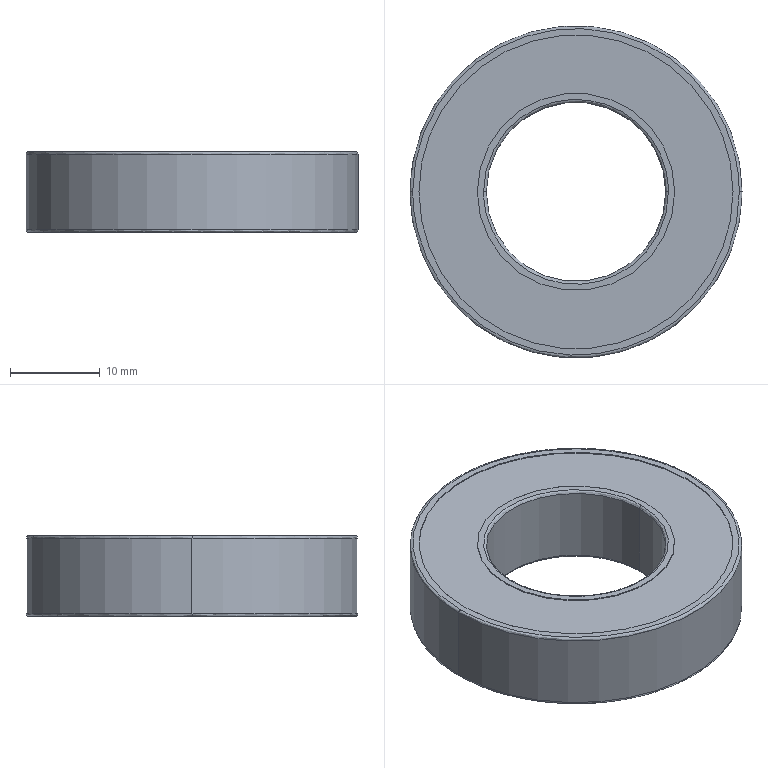Part | SolidWorks | features BaseBody 1 | 1 solid | 26 faces | box 37 x 37 x 9 mm | volume 6727 mm3 | cylinder 12 | spline 8 | plane 6 | commonest cylinder face diameters 22 x4 35 x4 20 x2 37 x2
STEP:
#1=CARTESIAN_POINT('',(-18.2,0.,-9.));
#2=VERTEX_POINT('',#1);
#3=CARTESIAN_POINT('',(18.2,0.,-9.));
#4=VERTEX_POINT('',#3);
#5=CARTESIAN_POINT('',(-18.2,0.,-9.));
#6=CARTESIAN_POINT('',(-18.2,-36.4,-9.));
#7=CARTESIAN_POINT('',(18.2,-36.4,-9.));
#8=CARTESIAN_POINT('',(18.2,0.,-9.));
#9=(BOUNDED_CURVE()B_SPLINE_CURVE(3,(#5,#6,#7,#8),.UNSPECIFIED.,.F.,.F.)B_SPLINE_CURVE_WITH_KNOTS((4,4),(0.,0.5),.UNSPECIFIED.)CURVE()GEOMETRIC_REPRESENTATION_ITEM()RATIONAL_B_SPLINE_CURVE((1.,0.3333,0.3333,1.))REPRESENTATION_ITEM(''));
#10=EDGE_CURVE('',#2,#4,#9,.T.);
#11=ORIENTED_EDGE('',*,*,#10,.T.);
#12=CARTESIAN_POINT('',(18.5,0.,-8.7));
#13=VERTEX_POINT('',#12);
#14=CARTESIAN_POINT('',(18.2,0.,-8.7));
#15=DIRECTION('',(0.,-1.,0.));
#16=DIRECTION('',(1.,0.,0.));
#17=AXIS2_PLACEMENT_3D('',#14,#15,#16);
#18=CIRCLE('',#17,0.3);
#19=EDGE_CURVE('',#4,#13,#18,.T.);
#20=ORIENTED_EDGE('',*,*,#19,.T.);
#21=CARTESIAN_POINT('',(-18.5,0.,-8.7));
#22=VERTEX_POINT('',#21);
#23=CARTESIAN_POINT('',(0.,0.,-8.7));
#24=DIRECTION('',(0.,0.,1.));
#25=DIRECTION('',(1.,0.,0.));
#26=AXIS2_PLACEMENT_3D('',#23,#24,#25);
#27=CIRCLE('',#26,18.5);
#28=EDGE_CURVE('',#22,#13,#27,.T.);
#29=ORIENTED_EDGE('',*,*,#28,.F.);
#30=CARTESIAN_POINT('',(-18.2,0.,-8.7));
#31=DIRECTION('',(0.,1.,0.));
#32=DIRECTION('',(-1.,0.,0.));
#33=AXIS2_PLACEMENT_3D('',#30,#31,#32);
#34=CIRCLE('',#33,0.3);
#35=EDGE_CURVE('',#2,#22,#34,.T.);
#36=ORIENTED_EDGE('',*,*,#35,.F.);
#37=EDGE_LOOP('',(#11,#20,#29,#36));
#38=FACE_OUTER_BOUND('',#37,.T.);
#39=CARTESIAN_POINT('',(18.2,0.,-9.));
#40=CARTESIAN_POINT('',(18.2,-36.4,-9.));
#41=CARTESIAN_POINT('',(-18.2,-36.4,-9.));
#42=CARTESIAN_POINT('',(-18.2,0.,-9.));
#43=CARTESIAN_POINT('',(18.376,0.,-9.));
#44=CARTESIAN_POINT('',(18.376,-36.751,-9.));
#45=CARTESIAN_POINT('',(-18.376,-36.751,-9.));
#46=CARTESIAN_POINT('',(-18.376,0.,-9.));
#47=CARTESIAN_POINT('',(18.5,0.,-8.876));
#48=CARTESIAN_POINT('',(18.5,-37.,-8.876));
#49=CARTESIAN_POINT('',(-18.5,-37.,-8.876));
#50=CARTESIAN_POINT('',(-18.5,0.,-8.876));
#51=CARTESIAN_POINT('',(18.5,0.,-8.7));
#52=CARTESIAN_POINT('',(18.5,-37.,-8.7));
#53=CARTESIAN_POINT('',(-18.5,-37.,-8.7));
#54=CARTESIAN_POINT('',(-18.5,0.,-8.7));
#55=(BOUNDED_SURFACE()B_SPLINE_SURFACE(3,3,((#39,#40,#41,#42),(#43,#44,#45,#46),(#47,#48,#49,#50),(#51,#52,#53,#54)),.UNSPECIFIED.,.F.,.F.,.F.)B_SPLINE_SURFACE_WITH_KNOTS((4,4),(4,4),(0.,1.),(0.,1.),.UNSPECIFIED.)GEOMETRIC_REPRESENTATION_ITEM()RATIONAL_B_SPLINE_SURFACE(((1.,0.3333,0.3333,1.),(0.8047,0.2682,0.2682,0.8047),(0.8047,0.2682,0.2682,0.8047),(1.,0.3333,0.3333,1.)))REPRESENTATION_ITEM('')SURFACE());
#56=ADVANCED_FACE('',(#38),#55,.T.);
#57=CARTESIAN_POINT('',(18.5,0.,-0.3));
#58=VERTEX_POINT('',#57);
#59=CARTESIAN_POINT('',(-18.5,0.,-0.3));
#60=VERTEX_POINT('',#59);
#61=CARTESIAN_POINT('',(0.,0.,-0.3));
#62=DIRECTION('',(0.,0.,-1.));
#63=DIRECTION('',(1.,0.,0.));
#64=AXIS2_PLACEMENT_3D('',#61,#62,#63);
#65=CIRCLE('',#64,18.5);
#66=EDGE_CURVE('',#58,#60,#65,.T.);
#67=ORIENTED_EDGE('',*,*,#66,.F.);
#68=CARTESIAN_POINT('',(18.2,0.,0.));
#69=VERTEX_POINT('',#68);
#70=CARTESIAN_POINT('',(18.2,0.,-0.3));
#71=DIRECTION('',(0.,-1.,0.));
#72=DIRECTION('',(1.,0.,0.));
#73=AXIS2_PLACEMENT_3D('',#70,#71,#72);
#74=CIRCLE('',#73,0.3);
#75=EDGE_CURVE('',#58,#69,#74,.T.);
#76=ORIENTED_EDGE('',*,*,#75,.T.);
#77=CARTESIAN_POINT('',(-18.2,0.,0.));
#78=VERTEX_POINT('',#77);
#79=CARTESIAN_POINT('',(18.2,0.,0.));
#80=CARTESIAN_POINT('',(18.2,-36.4,0.));
#81=CARTESIAN_POINT('',(-18.2,-36.4,0.));
#82=CARTESIAN_POINT('',(-18.2,0.,0.));
#83=(BOUNDED_CURVE()B_SPLINE_CURVE(3,(#79,#80,#81,#82),.UNSPECIFIED.,.F.,.F.)B_SPLINE_CURVE_WITH_KNOTS((4,4),(0.5,1.),.UNSPECIFIED.)CURVE()GEOMETRIC_REPRESENTATION_ITEM()RATIONAL_B_SPLINE_CURVE((1.,0.3333,0.3333,1.))REPRESENTATION_ITEM(''));
#84=EDGE_CURVE('',#69,#78,#83,.T.);
#85=ORIENTED_EDGE('',*,*,#84,.T.);
#86=CARTESIAN_POINT('',(-18.2,0.,-0.3));
#87=DIRECTION('',(0.,1.,0.));
#88=DIRECTION('',(-1.,0.,0.));
#89=AXIS2_PLACEMENT_3D('',#86,#87,#88);
#90=CIRCLE('',#89,0.3);
#91=EDGE_CURVE('',#60,#78,#90,.T.);
#92=ORIENTED_EDGE('',*,*,#91,.F.);
#93=EDGE_LOOP('',(#67,#76,#85,#92));
#94=FACE_OUTER_BOUND('',#93,.T.);
#95=CARTESIAN_POINT('',(18.5,0.,-0.3));
#96=CARTESIAN_POINT('',(18.5,-37.,-0.3));
#97=CARTESIAN_POINT('',(-18.5,-37.,-0.3));
#98=CARTESIAN_POINT('',(-18.5,0.,-0.3));
#99=CARTESIAN_POINT('',(18.5,0.,-0.1243));
#100=CARTESIAN_POINT('',(18.5,-37.,-0.1243));
#101=CARTESIAN_POINT('',(-18.5,-37.,-0.1243));
#102=CARTESIAN_POINT('',(-18.5,0.,-0.1243));
#103=CARTESIAN_POINT('',(18.376,0.,0.));
#104=CARTESIAN_POINT('',(18.376,-36.751,0.));
#105=CARTESIAN_POINT('',(-18.376,-36.751,0.));
#106=CARTESIAN_POINT('',(-18.376,0.,0.));
#107=CARTESIAN_POINT('',(18.2,0.,0.));
#108=CARTESIAN_POINT('',(18.2,-36.4,0.));
#109=CARTESIAN_POINT('',(-18.2,-36.4,0.));
#110=CARTESIAN_POINT('',(-18.2,0.,0.));
#111=(BOUNDED_SURFACE()B_SPLINE_SURFACE(3,3,((#95,#96,#97,#98),(#99,#100,#101,#102),(#103,#104,#105,#106),(#107,#108,#109,#110)),.UNSPECIFIED.,.F.,.F.,.F.)B_SPLINE_SURFACE_WITH_KNOTS((4,4),(4,4),(0.,1.),(0.,1.),.UNSPECIFIED.)GEOMETRIC_REPRESENTATION_ITEM()RATIONAL_B_SPLINE_SURFACE(((1.,0.3333,0.3333,1.),(0.8047,0.2682,0.2682,0.8047),(0.8047,0.2682,0.2682,0.8047),(1.,0.3333,0.3333,1.)))REPRESENTATION_ITEM('')SURFACE());
#112=ADVANCED_FACE('',(#94),#111,.T.);
#113=CARTESIAN_POINT('',(-10.,0.,-8.7));
#114=VERTEX_POINT('',#113);
#115=CARTESIAN_POINT('',(10.,0.,-8.7));
#116=VERTEX_POINT('',#115);
#117=CARTESIAN_POINT('',(0.,0.,-8.7));
#118=DIRECTION('',(0.,0.,1.));
#119=DIRECTION('',(-1.,0.,0.));
#120=AXIS2_PLACEMENT_3D('',#117,#118,#119);
#121=CIRCLE('',#120,10.);
#122=EDGE_CURVE('',#114,#116,#121,.T.);
#123=ORIENTED_EDGE('',*,*,#122,.T.);
#124=CARTESIAN_POINT('',(10.3,0.,-9.));
#125=VERTEX_POINT('',#124);
#126=CARTESIAN_POINT('',(10.3,0.,-8.7));
#127=DIRECTION('',(0.,-1.,0.));
#128=DIRECTION('',(1.,0.,0.));
#129=AXIS2_PLACEMENT_3D('',#126,#127,#128);
#130=CIRCLE('',#129,0.3);
#131=EDGE_CURVE('',#116,#125,#130,.T.);
#132=ORIENTED_EDGE('',*,*,#131,.T.);
#133=CARTESIAN_POINT('',(-10.3,0.,-9.));
#134=VERTEX_POINT('',#133);
#135=CARTESIAN_POINT('',(-10.3,0.,-9.));
#136=CARTESIAN_POINT('',(-10.3,-0.3149,-9.));
#137=CARTESIAN_POINT('',(-10.279,-0.7854,-9.));
#138=CARTESIAN_POINT('',(-10.216,-1.331,-9.));
#139=CARTESIAN_POINT('',(-10.175,-1.603,-9.));
#140=CARTESIAN_POINT('',(-10.152,-1.739,-9.));
#141=CARTESIAN_POINT('',(-10.142,-1.797,-9.));
#142=CARTESIAN_POINT('',(-10.135,-1.835,-9.));
#143=CARTESIAN_POINT('',(-10.132,-1.854,-9.));
#144=CARTESIAN_POINT('',(-10.067,-2.203,-9.));
#145=CARTESIAN_POINT('',(-9.953,-2.688,-9.));
#146=CARTESIAN_POINT('',(-9.778,-3.244,-9.));
#147=CARTESIAN_POINT('',(-9.681,-3.519,-9.));
#148=CARTESIAN_POINT('',(-9.637,-3.636,-9.));
#149=CARTESIAN_POINT('',(-9.607,-3.714,-9.));
#150=CARTESIAN_POINT('',(-9.593,-3.751,-9.));
#151=CARTESIAN_POINT('',(-9.449,-4.115,-9.));
#152=CARTESIAN_POINT('',(-9.233,-4.588,-9.));
#153=CARTESIAN_POINT('',(-8.941,-5.119,-9.));
#154=CARTESIAN_POINT('',(-8.807,-5.342,-9.));
#155=CARTESIAN_POINT('',(-8.715,-5.49,-9.));
#156=CARTESIAN_POINT('',(-8.67,-5.562,-9.));
#157=CARTESIAN_POINT('',(-8.232,-6.231,-9.));
#158=CARTESIAN_POINT('',(-7.786,-6.781,-9.));
#159=CARTESIAN_POINT('',(-7.032,-7.534,-9.));
#160=CARTESIAN_POINT('',(-6.638,-7.89,-9.));
#161=CARTESIAN_POINT('',(-6.147,-8.268,-9.));
#162=CARTESIAN_POINT('',(-5.93,-8.422,-9.));
#163=CARTESIAN_POINT('',(-5.784,-8.523,-9.));
#164=CARTESIAN_POINT('',(-5.709,-8.573,-9.));
#165=CARTESIAN_POINT('',(-5.345,-8.811,-9.));
#166=CARTESIAN_POINT('',(-4.896,-9.074,-9.));
#167=CARTESIAN_POINT('',(-4.351,-9.339,-9.));
#168=CARTESIAN_POINT('',(-4.073,-9.461,-9.));
#169=CARTESIAN_POINT('',(-3.953,-9.512,-9.));
#170=CARTESIAN_POINT('',(-3.872,-9.545,-9.));
#171=CARTESIAN_POINT('',(-3.83,-9.561,-9.));
#172=CARTESIAN_POINT('',(-3.481,-9.7,-9.));
#173=CARTESIAN_POINT('',(-3.008,-9.861,-9.));
#174=CARTESIAN_POINT('',(-2.445,-10.008,-9.));
#175=CARTESIAN_POINT('',(-2.161,-10.071,-9.));
#176=CARTESIAN_POINT('',(-2.018,-10.101,-9.));
#177=CARTESIAN_POINT('',(-1.956,-10.113,-9.));
#178=CARTESIAN_POINT('',(-1.915,-10.12,-9.));
#179=CARTESIAN_POINT('',(-1.894,-10.124,-9.));
#180=CARTESIAN_POINT('',(-1.255,-10.243,-9.));
#181=CARTESIAN_POINT('',(-0.6296,-10.3,-9.));
#182=CARTESIAN_POINT('',(0.3148,-10.3,-9.));
#183=CARTESIAN_POINT('',(0.7852,-10.279,-9.));
#184=CARTESIAN_POINT('',(1.331,-10.216,-9.));
#185=CARTESIAN_POINT('',(1.603,-10.175,-9.));
#186=CARTESIAN_POINT('',(1.739,-10.152,-9.));
#187=CARTESIAN_POINT('',(1.797,-10.142,-9.));
#188=CARTESIAN_POINT('',(1.835,-10.135,-9.));
#189=CARTESIAN_POINT('',(1.854,-10.132,-9.));
#190=CARTESIAN_POINT('',(2.203,-10.067,-9.));
#191=CARTESIAN_POINT('',(2.688,-9.953,-9.));
#192=CARTESIAN_POINT('',(3.244,-9.778,-9.));
#193=CARTESIAN_POINT('',(3.519,-9.681,-9.));
#194=CARTESIAN_POINT('',(3.636,-9.637,-9.));
#195=CARTESIAN_POINT('',(3.714,-9.607,-9.));
#196=CARTESIAN_POINT('',(3.751,-9.593,-9.));
#197=CARTESIAN_POINT('',(4.115,-9.449,-9.));
#198=CARTESIAN_POINT('',(4.588,-9.233,-9.));
#199=CARTESIAN_POINT('',(5.119,-8.941,-9.));
#200=CARTESIAN_POINT('',(5.342,-8.807,-9.));
#201=CARTESIAN_POINT('',(5.49,-8.715,-9.));
#202=CARTESIAN_POINT('',(5.562,-8.67,-9.));
#203=CARTESIAN_POINT('',(6.231,-8.232,-9.));
#204=CARTESIAN_POINT('',(6.781,-7.786,-9.));
#205=CARTESIAN_POINT('',(7.534,-7.032,-9.));
#206=CARTESIAN_POINT('',(7.89,-6.638,-9.));
#207=CARTESIAN_POINT('',(8.268,-6.147,-9.));
#208=CARTESIAN_POINT('',(8.422,-5.93,-9.));
#209=CARTESIAN_POINT('',(8.523,-5.784,-9.));
#210=CARTESIAN_POINT('',(8.573,-5.709,-9.));
#211=CARTESIAN_POINT('',(8.811,-5.345,-9.));
#212=CARTESIAN_POINT('',(9.074,-4.896,-9.));
#213=CARTESIAN_POINT('',(9.339,-4.351,-9.));
#214=CARTESIAN_POINT('',(9.461,-4.073,-9.));
#215=CARTESIAN_POINT('',(9.512,-3.953,-9.));
#216=CARTESIAN_POINT('',(9.545,-3.872,-9.));
#217=CARTESIAN_POINT('',(9.561,-3.83,-9.));
#218=CARTESIAN_POINT('',(9.7,-3.481,-9.));
#219=CARTESIAN_POINT('',(9.861,-3.008,-9.));
#220=CARTESIAN_POINT('',(10.008,-2.445,-9.));
#221=CARTESIAN_POINT('',(10.071,-2.161,-9.));
#222=CARTESIAN_POINT('',(10.101,-2.018,-9.));
#223=CARTESIAN_POINT('',(10.113,-1.956,-9.));
#224=CARTESIAN_POINT('',(10.12,-1.915,-9.));
#225=CARTESIAN_POINT('',(10.124,-1.894,-9.));
#226=CARTESIAN_POINT('',(10.243,-1.255,-9.));
#227=CARTESIAN_POINT('',(10.3,-0.6296,-9.));
#228=CARTESIAN_POINT('',(10.3,0.,-9.));
#229=B_SPLINE_CURVE_WITH_KNOTS('',3,(#135,#136,#137,#138,#139,#140,#141,#142,#143,#144,#145,#146,#147,#148,#149,#150,#151,#152,#153,#154,#155,#156,#157,#158,#159,#160,#161,#162,#163,#164,#165,#166,#167,#168,#169,#170,#171,#172,#173,#174,#175,#176,#177,#178,#179,#180,#181,#182,#183,#184,#185,#186,#187,#188,#189,#190,#191,#192,#193,#194,#195,#196,#197,#198,#199,#200,#201,#202,#203,#204,#205,#206,#207,#208,#209,#210,#211,#212,#213,#214,#215,#216,#217,#218,#219,#220,#221,#222,#223,#224,#225,#226,#227,#228),.UNSPECIFIED.,.F.,.F.,(4,1,1,1,1,2,2,1,1,1,2,2,1,1,2,2,2,1,1,2,2,1,1,1,2,2,1,1,1,1,2,2,2,1,1,1,1,2,2,1,1,1,2,2,1,1,2,2,2,1,1,2,2,1,1,1,2,2,1,1,1,1,2,2,4),(0.,0.01563,0.02344,0.02734,0.0293,0.03027,0.03125,0.04688,0.05469,0.05859,0.06055,0.0625,0.07813,0.08594,0.08984,0.09375,0.125,0.1406,0.1484,0.1523,0.1563,0.1719,0.1797,0.1836,0.1855,0.1875,0.2031,0.2109,0.2148,0.2168,0.2178,0.2188,0.25,0.2656,0.2734,0.2773,0.2793,0.2803,0.2813,0.2969,0.3047,0.3086,0.3105,0.3125,0.3281,0.3359,0.3398,0.3438,0.375,0.3906,0.3984,0.4023,0.4063,0.4219,0.4297,0.4336,0.4355,0.4375,0.4531,0.4609,0.4648,0.4668,0.4678,0.4688,0.5),.UNSPECIFIED.);
#230=EDGE_CURVE('',#134,#125,#229,.T.);
#231=ORIENTED_EDGE('',*,*,#230,.F.);
#232=CARTESIAN_POINT('',(-10.3,0.,-8.7));
#233=DIRECTION('',(0.,1.,0.));
#234=DIRECTION('',(-1.,0.,0.));
#235=AXIS2_PLACEMENT_3D('',#232,#233,#234);
#236=CIRCLE('',#235,0.3);
#237=EDGE_CURVE('',#114,#134,#236,.T.);
#238=ORIENTED_EDGE('',*,*,#237,.F.);
#239=EDGE_LOOP('',(#123,#132,#231,#238));
#240=FACE_OUTER_BOUND('',#239,.T.);
#241=CARTESIAN_POINT('',(10.,0.,-8.7));
#242=CARTESIAN_POINT('',(10.,-20.,-8.7));
#243=CARTESIAN_POINT('',(-10.,-20.,-8.7));
#244=CARTESIAN_POINT('',(-10.,0.,-8.7));
#245=CARTESIAN_POINT('',(10.,0.,-8.876));
#246=CARTESIAN_POINT('',(10.,-20.,-8.876));
#247=CARTESIAN_POINT('',(-10.,-20.,-8.876));
#248=CARTESIAN_POINT('',(-10.,0.,-8.876));
#249=CARTESIAN_POINT('',(10.124,0.,-9.));
#250=CARTESIAN_POINT('',(10.124,-20.249,-9.));
#251=CARTESIAN_POINT('',(-10.124,-20.249,-9.));
#252=CARTESIAN_POINT('',(-10.124,0.,-9.));
#253=CARTESIAN_POINT('',(10.3,0.,-9.));
#254=CARTESIAN_POINT('',(10.3,-20.6,-9.));
#255=CARTESIAN_POINT('',(-10.3,-20.6,-9.));
#256=CARTESIAN_POINT('',(-10.3,0.,-9.));
#257=(BOUNDED_SURFACE()B_SPLINE_SURFACE(3,3,((#241,#242,#243,#244),(#245,#246,#247,#248),(#249,#250,#251,#252),(#253,#254,#255,#256)),.UNSPECIFIED.,.F.,.F.,.F.)B_SPLINE_SURFACE_WITH_KNOTS((4,4),(4,4),(0.,1.),(0.,1.),.UNSPECIFIED.)GEOMETRIC_REPRESENTATION_ITEM()RATIONAL_B_SPLINE_SURFACE(((1.,0.3333,0.3333,1.),(0.8047,0.2682,0.2682,0.8047),(0.8047,0.2682,0.2682,0.8047),(1.,0.3333,0.3333,1.)))REPRESENTATION_ITEM('')SURFACE());
#258=ADVANCED_FACE('',(#240),#257,.T.);
#259=CARTESIAN_POINT('',(10.3,0.,0.));
#260=VERTEX_POINT('',#259);
#261=CARTESIAN_POINT('',(-10.3,0.,0.));
#262=VERTEX_POINT('',#261);
#263=CARTESIAN_POINT('',(10.3,0.,0.));
#264=CARTESIAN_POINT('',(10.3,-0.3148,0.));
#265=CARTESIAN_POINT('',(10.279,-0.7852,0.));
#266=CARTESIAN_POINT('',(10.216,-1.331,0.));
#267=CARTESIAN_POINT('',(10.175,-1.603,0.));
#268=CARTESIAN_POINT('',(10.152,-1.739,0.));
#269=CARTESIAN_POINT('',(10.142,-1.797,0.));
#270=CARTESIAN_POINT('',(10.135,-1.835,0.));
#271=CARTESIAN_POINT('',(10.132,-1.854,0.));
#272=CARTESIAN_POINT('',(10.067,-2.203,0.));
#273=CARTESIAN_POINT('',(9.953,-2.688,0.));
#274=CARTESIAN_POINT('',(9.778,-3.244,0.));
#275=CARTESIAN_POINT('',(9.681,-3.519,0.));
#276=CARTESIAN_POINT('',(9.637,-3.636,0.));
#277=CARTESIAN_POINT('',(9.607,-3.714,0.));
#278=CARTESIAN_POINT('',(9.593,-3.751,0.));
#279=CARTESIAN_POINT('',(9.449,-4.115,0.));
#280=CARTESIAN_POINT('',(9.233,-4.588,0.));
#281=CARTESIAN_POINT('',(8.941,-5.119,0.));
#282=CARTESIAN_POINT('',(8.807,-5.342,0.));
#283=CARTESIAN_POINT('',(8.715,-5.49,0.));
#284=CARTESIAN_POINT('',(8.67,-5.562,0.));
#285=CARTESIAN_POINT('',(8.232,-6.231,0.));
#286=CARTESIAN_POINT('',(7.786,-6.781,0.));
#287=CARTESIAN_POINT('',(7.032,-7.534,0.));
#288=CARTESIAN_POINT('',(6.638,-7.89,0.));
#289=CARTESIAN_POINT('',(6.147,-8.268,0.));
#290=CARTESIAN_POINT('',(5.93,-8.422,0.));
#291=CARTESIAN_POINT('',(5.784,-8.523,0.));
#292=CARTESIAN_POINT('',(5.709,-8.573,0.));
#293=CARTESIAN_POINT('',(5.345,-8.811,0.));
#294=CARTESIAN_POINT('',(4.896,-9.074,0.));
#295=CARTESIAN_POINT('',(4.351,-9.339,0.));
#296=CARTESIAN_POINT('',(4.073,-9.461,0.));
#297=CARTESIAN_POINT('',(3.953,-9.512,0.));
#298=CARTESIAN_POINT('',(3.872,-9.545,0.));
#299=CARTESIAN_POINT('',(3.83,-9.561,0.));
#300=CARTESIAN_POINT('',(3.481,-9.7,0.));
#301=CARTESIAN_POINT('',(3.008,-9.861,0.));
#302=CARTESIAN_POINT('',(2.445,-10.008,0.));
#303=CARTESIAN_POINT('',(2.161,-10.071,0.));
#304=CARTESIAN_POINT('',(2.018,-10.101,0.));
#305=CARTESIAN_POINT('',(1.956,-10.113,0.));
#306=CARTESIAN_POINT('',(1.915,-10.12,0.));
#307=CARTESIAN_POINT('',(1.894,-10.124,0.));
#308=CARTESIAN_POINT('',(1.255,-10.243,0.));
#309=CARTESIAN_POINT('',(0.6296,-10.3,0.));
#310=CARTESIAN_POINT('',(-0.3148,-10.3,0.));
#311=CARTESIAN_POINT('',(-0.7852,-10.279,0.));
#312=CARTESIAN_POINT('',(-1.331,-10.216,0.));
#313=CARTESIAN_POINT('',(-1.603,-10.175,0.));
#314=CARTESIAN_POINT('',(-1.739,-10.152,0.));
#315=CARTESIAN_POINT('',(-1.797,-10.142,0.));
#316=CARTESIAN_POINT('',(-1.835,-10.135,0.));
#317=CARTESIAN_POINT('',(-1.854,-10.132,0.));
#318=CARTESIAN_POINT('',(-2.203,-10.067,0.));
#319=CARTESIAN_POINT('',(-2.688,-9.953,0.));
#320=CARTESIAN_POINT('',(-3.244,-9.778,0.));
#321=CARTESIAN_POINT('',(-3.519,-9.681,0.));
#322=CARTESIAN_POINT('',(-3.636,-9.637,0.));
#323=CARTESIAN_POINT('',(-3.714,-9.607,0.));
#324=CARTESIAN_POINT('',(-3.751,-9.593,0.));
#325=CARTESIAN_POINT('',(-4.115,-9.449,0.));
#326=CARTESIAN_POINT('',(-4.588,-9.233,0.));
#327=CARTESIAN_POINT('',(-5.119,-8.941,0.));
#328=CARTESIAN_POINT('',(-5.342,-8.807,0.));
#329=CARTESIAN_POINT('',(-5.49,-8.715,0.));
#330=CARTESIAN_POINT('',(-5.562,-8.67,0.));
#331=CARTESIAN_POINT('',(-6.231,-8.232,0.));
#332=CARTESIAN_POINT('',(-6.781,-7.786,0.));
#333=CARTESIAN_POINT('',(-7.534,-7.032,0.));
#334=CARTESIAN_POINT('',(-7.89,-6.638,0.));
#335=CARTESIAN_POINT('',(-8.268,-6.147,0.));
#336=CARTESIAN_POINT('',(-8.422,-5.93,0.));
#337=CARTESIAN_POINT('',(-8.523,-5.784,0.));
#338=CARTESIAN_POINT('',(-8.573,-5.709,0.));
#339=CARTESIAN_POINT('',(-8.811,-5.345,0.));
#340=CARTESIAN_POINT('',(-9.074,-4.896,0.));
#341=CARTESIAN_POINT('',(-9.339,-4.351,0.));
#342=CARTESIAN_POINT('',(-9.461,-4.073,0.));
#343=CARTESIAN_POINT('',(-9.512,-3.953,0.));
#344=CARTESIAN_POINT('',(-9.545,-3.872,0.));
#345=CARTESIAN_POINT('',(-9.561,-3.83,0.));
#346=CARTESIAN_POINT('',(-9.7,-3.481,0.));
#347=CARTESIAN_POINT('',(-9.861,-3.008,0.));
#348=CARTESIAN_POINT('',(-10.008,-2.445,0.));
#349=CARTESIAN_POINT('',(-10.071,-2.161,0.));
#350=CARTESIAN_POINT('',(-10.101,-2.018,0.));
#351=CARTESIAN_POINT('',(-10.113,-1.956,0.));
#352=CARTESIAN_POINT('',(-10.12,-1.915,0.));
#353=CARTESIAN_POINT('',(-10.124,-1.894,0.));
#354=CARTESIAN_POINT('',(-10.243,-1.255,0.));
#355=CARTESIAN_POINT('',(-10.3,-0.6302,0.));
#356=CARTESIAN_POINT('',(-10.3,0.,0.));
#357=B_SPLINE_CURVE_WITH_KNOTS('',3,(#263,#264,#265,#266,#267,#268,#269,#270,#271,#272,#273,#274,#275,#276,#277,#278,#279,#280,#281,#282,#283,#284,#285,#286,#287,#288,#289,#290,#291,#292,#293,#294,#295,#296,#297,#298,#299,#300,#301,#302,#303,#304,#305,#306,#307,#308,#309,#310,#311,#312,#313,#314,#315,#316,#317,#318,#319,#320,#321,#322,#323,#324,#325,#326,#327,#328,#329,#330,#331,#332,#333,#334,#335,#336,#337,#338,#339,#340,#341,#342,#343,#344,#345,#346,#347,#348,#349,#350,#351,#352,#353,#354,#355,#356),.UNSPECIFIED.,.F.,.F.,(4,1,1,1,1,2,2,1,1,1,2,2,1,1,2,2,2,1,1,2,2,1,1,1,2,2,1,1,1,1,2,2,2,1,1,1,1,2,2,1,1,1,2,2,1,1,2,2,2,1,1,2,2,1,1,1,2,2,1,1,1,1,2,2,4),(0.5,0.5156,0.5234,0.5273,0.5293,0.5303,0.5313,0.5469,0.5547,0.5586,0.5605,0.5625,0.5781,0.5859,0.5898,0.5938,0.625,0.6406,0.6484,0.6523,0.6563,0.6719,0.6797,0.6836,0.6855,0.6875,0.7031,0.7109,0.7148,0.7168,0.7178,0.7188,0.75,0.7656,0.7734,0.7773,0.7793,0.7803,0.7813,0.7969,0.8047,0.8086,0.8105,0.8125,0.8281,0.8359,0.8398,0.8438,0.875,0.8906,0.8984,0.9023,0.9063,0.9219,0.9297,0.9336,0.9355,0.9375,0.9531,0.9609,0.9648,0.9668,0.9678,0.9688,1.),.UNSPECIFIED.);
#358=EDGE_CURVE('',#260,#262,#357,.T.);
#359=ORIENTED_EDGE('',*,*,#358,.F.);
#360=CARTESIAN_POINT('',(10.,0.,-0.3));
#361=VERTEX_POINT('',#360);
#362=CARTESIAN_POINT('',(10.3,0.,-0.3));
#363=DIRECTION('',(0.,-1.,0.));
#364=DIRECTION('',(1.,0.,0.));
#365=AXIS2_PLACEMENT_3D('',#362,#363,#364);
#366=CIRCLE('',#365,0.3);
#367=EDGE_CURVE('',#260,#361,#366,.T.);
#368=ORIENTED_EDGE('',*,*,#367,.T.);
#369=CARTESIAN_POINT('',(-10.,0.,-0.3));
#370=VERTEX_POINT('',#369);
#371=CARTESIAN_POINT('',(0.,0.,-0.3));
#372=DIRECTION('',(0.,0.,-1.));
#373=DIRECTION('',(-1.,0.,0.));
#374=AXIS2_PLACEMENT_3D('',#371,#372,#373);
#375=CIRCLE('',#374,10.);
#376=EDGE_CURVE('',#361,#370,#375,.T.);
#377=ORIENTED_EDGE('',*,*,#376,.T.);
#378=CARTESIAN_POINT('',(-10.3,0.,-0.3));
#379=DIRECTION('',(0.,1.,0.));
#380=DIRECTION('',(-1.,0.,0.));
#381=AXIS2_PLACEMENT_3D('',#378,#379,#380);
#382=CIRCLE('',#381,0.3);
#383=EDGE_CURVE('',#262,#370,#382,.T.);
#384=ORIENTED_EDGE('',*,*,#383,.F.);
#385=EDGE_LOOP('',(#359,#368,#377,#384));
#386=FACE_OUTER_BOUND('',#385,.T.);
#387=CARTESIAN_POINT('',(10.3,0.,0.));
#388=CARTESIAN_POINT('',(10.3,-20.6,0.));
#389=CARTESIAN_POINT('',(-10.3,-20.6,0.));
#390=CARTESIAN_POINT('',(-10.3,0.,0.));
#391=CARTESIAN_POINT('',(10.124,0.,0.));
#392=CARTESIAN_POINT('',(10.124,-20.249,0.));
#393=CARTESIAN_POINT('',(-10.124,-20.249,0.));
#394=CARTESIAN_POINT('',(-10.124,0.,0.));
#395=CARTESIAN_POINT('',(10.,0.,-0.1243));
#396=CARTESIAN_POINT('',(10.,-20.,-0.1243));
#397=CARTESIAN_POINT('',(-10.,-20.,-0.1243));
#398=CARTESIAN_POINT('',(-10.,0.,-0.1243));
#399=CARTESIAN_POINT('',(10.,0.,-0.3));
#400=CARTESIAN_POINT('',(10.,-20.,-0.3));
#401=CARTESIAN_POINT('',(-10.,-20.,-0.3));
#402=CARTESIAN_POINT('',(-10.,0.,-0.3));
#403=(BOUNDED_SURFACE()B_SPLINE_SURFACE(3,3,((#387,#388,#389,#390),(#391,#392,#393,#394),(#395,#396,#397,#398),(#399,#400,#401,#402)),.UNSPECIFIED.,.F.,.F.,.F.)B_SPLINE_SURFACE_WITH_KNOTS((4,4),(4,4),(0.,1.),(0.,1.),.UNSPECIFIED.)GEOMETRIC_REPRESENTATION_ITEM()RATIONAL_B_SPLINE_SURFACE(((1.,0.3333,0.3333,1.),(0.8047,0.2682,0.2682,0.8047),(0.8047,0.2682,0.2682,0.8047),(1.,0.3333,0.3333,1.)))REPRESENTATION_ITEM('')SURFACE());
#404=ADVANCED_FACE('',(#386),#403,.T.);
#405=CARTESIAN_POINT('',(0.,0.,-8.7));
#406=DIRECTION('',(0.,0.,1.));
#407=DIRECTION('',(1.,0.,0.));
#408=AXIS2_PLACEMENT_3D('',#405,#406,#407);
#409=CIRCLE('',#408,18.5);
#410=EDGE_CURVE('',#13,#22,#409,.T.);
#411=ORIENTED_EDGE('',*,*,#410,.T.);
#412=CARTESIAN_POINT('',(-18.5,0.,-9.));
#413=DIRECTION('',(0.,0.,1.));
#414=VECTOR('',#413,1000.);
#415=LINE('',#412,#414);
#416=EDGE_CURVE('',#22,#60,#415,.T.);
#417=ORIENTED_EDGE('',*,*,#416,.T.);
#418=CARTESIAN_POINT('',(0.,0.,-0.3));
#419=DIRECTION('',(0.,0.,-1.));
#420=DIRECTION('',(1.,0.,0.));
#421=AXIS2_PLACEMENT_3D('',#418,#419,#420);
#422=CIRCLE('',#421,18.5);
#423=EDGE_CURVE('',#60,#58,#422,.T.);
#424=ORIENTED_EDGE('',*,*,#423,.T.);
#425=CARTESIAN_POINT('',(18.5,0.,-9.));
#426=DIRECTION('',(0.,0.,1.));
#427=VECTOR('',#426,1000.);
#428=LINE('',#425,#427);
#429=EDGE_CURVE('',#13,#58,#428,.T.);
#430=ORIENTED_EDGE('',*,*,#429,.F.);
#431=EDGE_LOOP('',(#411,#417,#424,#430));
#432=FACE_OUTER_BOUND('',#431,.T.);
#433=CARTESIAN_POINT('',(0.,0.,-9.));
#434=DIRECTION('',(0.,0.,1.));
#435=DIRECTION('',(1.,0.,0.));
#436=AXIS2_PLACEMENT_3D('',#433,#434,#435);
#437=CYLINDRICAL_SURFACE('',#436,18.5);
#438=ADVANCED_FACE('',(#432),#437,.T.);
#439=CARTESIAN_POINT('',(-17.5,0.,-9.));
#440=VERTEX_POINT('',#439);
#441=CARTESIAN_POINT('',(17.5,0.,-9.));
#442=VERTEX_POINT('',#441);
#443=CARTESIAN_POINT('',(0.,0.,-9.));
#444=DIRECTION('',(0.,0.,1.));
#445=DIRECTION('',(1.,0.,0.));
#446=AXIS2_PLACEMENT_3D('',#443,#444,#445);
#447=CIRCLE('',#446,17.5);
#448=EDGE_CURVE('',#440,#442,#447,.T.);
#449=ORIENTED_EDGE('',*,*,#448,.F.);
#450=CARTESIAN_POINT('',(-17.5,0.,-8.9));
#451=VERTEX_POINT('',#450);
#452=CARTESIAN_POINT('',(-17.5,0.,-9.));
#453=DIRECTION('',(0.,0.,1.));
#454=VECTOR('',#453,1000.);
#455=LINE('',#452,#454);
#456=EDGE_CURVE('',#440,#451,#455,.T.);
#457=ORIENTED_EDGE('',*,*,#456,.T.);
#458=CARTESIAN_POINT('',(17.5,0.,-8.9));
#459=VERTEX_POINT('',#458);
#460=CARTESIAN_POINT('',(0.,0.,-8.9));
#461=DIRECTION('',(0.,0.,-1.));
#462=DIRECTION('',(1.,0.,0.));
#463=AXIS2_PLACEMENT_3D('',#460,#461,#462);
#464=CIRCLE('',#463,17.5);
#465=EDGE_CURVE('',#459,#451,#464,.T.);
#466=ORIENTED_EDGE('',*,*,#465,.F.);
#467=CARTESIAN_POINT('',(17.5,0.,-9.));
#468=DIRECTION('',(0.,0.,1.));
#469=VECTOR('',#468,1000.);
#470=LINE('',#467,#469);
#471=EDGE_CURVE('',#442,#459,#470,.T.);
#472=ORIENTED_EDGE('',*,*,#471,.F.);
#473=EDGE_LOOP('',(#449,#457,#466,#472));
#474=FACE_OUTER_BOUND('',#473,.T.);
#475=CARTESIAN_POINT('',(0.,0.,-9.));
#476=DIRECTION('',(0.,0.,1.));
#477=DIRECTION('',(1.,0.,0.));
#478=AXIS2_PLACEMENT_3D('',#475,#476,#477);
#479=CYLINDRICAL_SURFACE('',#478,17.5);
#480=ADVANCED_FACE('',(#474),#479,.F.);
#481=CARTESIAN_POINT('',(-17.5,0.,-0.1));
#482=VERTEX_POINT('',#481);
#483=CARTESIAN_POINT('',(17.5,0.,-0.1));
#484=VERTEX_POINT('',#483);
#485=CARTESIAN_POINT('',(0.,0.,-0.1));
#486=DIRECTION('',(0.,0.,1.));
#487=DIRECTION('',(1.,0.,0.));
#488=AXIS2_PLACEMENT_3D('',#485,#486,#487);
#489=CIRCLE('',#488,17.5);
#490=EDGE_CURVE('',#482,#484,#489,.T.);
#491=ORIENTED_EDGE('',*,*,#490,.F.);
#492=CARTESIAN_POINT('',(-17.5,0.,0.));
#493=VERTEX_POINT('',#492);
#494=CARTESIAN_POINT('',(-17.5,0.,-9.));
#495=DIRECTION('',(0.,0.,1.));
#496=VECTOR('',#495,1000.);
#497=LINE('',#494,#496);
#498=EDGE_CURVE('',#482,#493,#497,.T.);
#499=ORIENTED_EDGE('',*,*,#498,.T.);
#500=CARTESIAN_POINT('',(17.5,0.,0.));
#501=VERTEX_POINT('',#500);
#502=CARTESIAN_POINT('',(0.,0.,0.));
#503=DIRECTION('',(0.,0.,-1.));
#504=DIRECTION('',(1.,0.,0.));
#505=AXIS2_PLACEMENT_3D('',#502,#503,#504);
#506=CIRCLE('',#505,17.5);
#507=EDGE_CURVE('',#501,#493,#506,.T.);
#508=ORIENTED_EDGE('',*,*,#507,.F.);
#509=CARTESIAN_POINT('',(17.5,0.,-9.));
#510=DIRECTION('',(0.,0.,1.));
#511=VECTOR('',#510,1000.);
#512=LINE('',#509,#511);
#513=EDGE_CURVE('',#484,#501,#512,.T.);
#514=ORIENTED_EDGE('',*,*,#513,.F.);
#515=EDGE_LOOP('',(#491,#499,#508,#514));
#516=FACE_OUTER_BOUND('',#515,.T.);
#517=CARTESIAN_POINT('',(0.,0.,-9.));
#518=DIRECTION('',(0.,0.,1.));
#519=DIRECTION('',(1.,0.,0.));
#520=AXIS2_PLACEMENT_3D('',#517,#518,#519);
#521=CYLINDRICAL_SURFACE('',#520,17.5);
#522=ADVANCED_FACE('',(#516),#521,.F.);
#523=CARTESIAN_POINT('',(11.,0.,-9.));
#524=VERTEX_POINT('',#523);
#525=CARTESIAN_POINT('',(-11.,0.,-9.));
#526=VERTEX_POINT('',#525);
#527=CARTESIAN_POINT('',(0.,0.,-9.));
#528=DIRECTION('',(0.,0.,1.));
#529=DIRECTION('',(1.,0.,0.));
#530=AXIS2_PLACEMENT_3D('',#527,#528,#529);
#531=CIRCLE('',#530,11.);
#532=EDGE_CURVE('',#524,#526,#531,.T.);
#533=ORIENTED_EDGE('',*,*,#532,.T.);
#534=CARTESIAN_POINT('',(-11.,0.,-8.9));
#535=VERTEX_POINT('',#534);
#536=CARTESIAN_POINT('',(-11.,0.,-9.));
#537=DIRECTION('',(0.,0.,1.));
#538=VECTOR('',#537,1000.);
#539=LINE('',#536,#538);
#540=EDGE_CURVE('',#526,#535,#539,.T.);
#541=ORIENTED_EDGE('',*,*,#540,.T.);
#542=CARTESIAN_POINT('',(11.,0.,-8.9));
#543=VERTEX_POINT('',#542);
#544=CARTESIAN_POINT('',(0.,0.,-8.9));
#545=DIRECTION('',(0.,0.,1.));
#546=DIRECTION('',(1.,0.,0.));
#547=AXIS2_PLACEMENT_3D('',#544,#545,#546);
#548=CIRCLE('',#547,11.);
#549=EDGE_CURVE('',#543,#535,#548,.T.);
#550=ORIENTED_EDGE('',*,*,#549,.F.);
#551=CARTESIAN_POINT('',(11.,0.,-9.));
#552=DIRECTION('',(0.,0.,1.));
#553=VECTOR('',#552,1000.);
#554=LINE('',#551,#553);
#555=EDGE_CURVE('',#524,#543,#554,.T.);
#556=ORIENTED_EDGE('',*,*,#555,.F.);
#557=EDGE_LOOP('',(#533,#541,#550,#556));
#558=FACE_OUTER_BOUND('',#557,.T.);
#559=CARTESIAN_POINT('',(0.,0.,-9.));
#560=DIRECTION('',(0.,0.,1.));
#561=DIRECTION('',(1.,0.,0.));
#562=AXIS2_PLACEMENT_3D('',#559,#560,#561);
#563=CYLINDRICAL_SURFACE('',#562,11.);
#564=ADVANCED_FACE('',(#558),#563,.T.);
#565=CARTESIAN_POINT('',(-11.,0.,-0.1));
#566=VERTEX_POINT('',#565);
#567=CARTESIAN_POINT('',(11.,0.,-0.1));
#568=VERTEX_POINT('',#567);
#569=CARTESIAN_POINT('',(0.,0.,-0.1));
#570=DIRECTION('',(0.,0.,-1.));
#571=DIRECTION('',(1.,0.,0.));
#572=AXIS2_PLACEMENT_3D('',#569,#570,#571);
#573=CIRCLE('',#572,11.);
#574=EDGE_CURVE('',#566,#568,#573,.T.);
#575=ORIENTED_EDGE('',*,*,#574,.F.);
#576=CARTESIAN_POINT('',(-11.,0.,0.));
#577=VERTEX_POINT('',#576);
#578=CARTESIAN_POINT('',(-11.,0.,-9.));
#579=DIRECTION('',(0.,0.,1.));
#580=VECTOR('',#579,1000.);
#581=LINE('',#578,#580);
#582=EDGE_CURVE('',#566,#577,#581,.T.);
#583=ORIENTED_EDGE('',*,*,#582,.T.);
#584=CARTESIAN_POINT('',(11.,0.,0.));
#585=VERTEX_POINT('',#584);
#586=CARTESIAN_POINT('',(0.,0.,0.));
#587=DIRECTION('',(0.,0.,-1.));
#588=DIRECTION('',(1.,0.,0.));
#589=AXIS2_PLACEMENT_3D('',#586,#587,#588);
#590=CIRCLE('',#589,11.);
#591=EDGE_CURVE('',#577,#585,#590,.T.);
#592=ORIENTED_EDGE('',*,*,#591,.T.);
#593=CARTESIAN_POINT('',(11.,0.,-9.));
#594=DIRECTION('',(0.,0.,1.));
#595=VECTOR('',#594,1000.);
#596=LINE('',#593,#595);
#597=EDGE_CURVE('',#568,#585,#596,.T.);
#598=ORIENTED_EDGE('',*,*,#597,.F.);
#599=EDGE_LOOP('',(#575,#583,#592,#598));
#600=FACE_OUTER_BOUND('',#599,.T.);
#601=CARTESIAN_POINT('',(0.,0.,-9.));
#602=DIRECTION('',(0.,0.,1.));
#603=DIRECTION('',(1.,0.,0.));
#604=AXIS2_PLACEMENT_3D('',#601,#602,#603);
#605=CYLINDRICAL_SURFACE('',#604,11.);
#606=ADVANCED_FACE('',(#600),#605,.T.);
#607=ORIENTED_EDGE('',*,*,#122,.F.);
#608=CARTESIAN_POINT('',(-10.,0.,-9.));
#609=DIRECTION('',(0.,0.,1.));
#610=VECTOR('',#609,1000.);
#611=LINE('',#608,#610);
#612=EDGE_CURVE('',#114,#370,#611,.T.);
#613=ORIENTED_EDGE('',*,*,#612,.T.);
#614=ORIENTED_EDGE('',*,*,#376,.F.);
#615=CARTESIAN_POINT('',(10.,0.,-9.));
#616=DIRECTION('',(0.,0.,1.));
#617=VECTOR('',#616,1000.);
#618=LINE('',#615,#617);
#619=EDGE_CURVE('',#116,#361,#618,.T.);
#620=ORIENTED_EDGE('',*,*,#619,.F.);
#621=EDGE_LOOP('',(#607,#613,#614,#620));
#622=FACE_OUTER_BOUND('',#621,.T.);
#623=CARTESIAN_POINT('',(0.,0.,-9.));
#624=DIRECTION('',(0.,0.,1.));
#625=DIRECTION('',(1.,0.,0.));
#626=AXIS2_PLACEMENT_3D('',#623,#624,#625);
#627=CYLINDRICAL_SURFACE('',#626,10.);
#628=ADVANCED_FACE('',(#622),#627,.F.);
#629=ORIENTED_EDGE('',*,*,#416,.F.);
#630=ORIENTED_EDGE('',*,*,#28,.T.);
#631=ORIENTED_EDGE('',*,*,#429,.T.);
#632=ORIENTED_EDGE('',*,*,#66,.T.);
#633=EDGE_LOOP('',(#629,#630,#631,#632));
#634=FACE_OUTER_BOUND('',#633,.T.);
#635=CARTESIAN_POINT('',(0.,0.,-9.));
#636=DIRECTION('',(0.,0.,1.));
#637=DIRECTION('',(1.,0.,0.));
#638=AXIS2_PLACEMENT_3D('',#635,#636,#637);
#639=CYLINDRICAL_SURFACE('',#638,18.5);
#640=ADVANCED_FACE('',(#634),#639,.T.);
#641=ORIENTED_EDGE('',*,*,#19,.F.);
#642=CARTESIAN_POINT('',(18.2,0.,-9.));
#643=CARTESIAN_POINT('',(18.2,36.4,-9.));
#644=CARTESIAN_POINT('',(-18.2,36.4,-9.));
#645=CARTESIAN_POINT('',(-18.2,0.,-9.));
#646=(BOUNDED_CURVE()B_SPLINE_CURVE(3,(#642,#643,#644,#645),.UNSPECIFIED.,.F.,.F.)B_SPLINE_CURVE_WITH_KNOTS((4,4),(0.5,1.),.UNSPECIFIED.)CURVE()GEOMETRIC_REPRESENTATION_ITEM()RATIONAL_B_SPLINE_CURVE((1.,0.3333,0.3333,1.))REPRESENTATION_ITEM(''));
#647=EDGE_CURVE('',#4,#2,#646,.T.);
#648=ORIENTED_EDGE('',*,*,#647,.T.);
#649=ORIENTED_EDGE('',*,*,#35,.T.);
#650=ORIENTED_EDGE('',*,*,#410,.F.);
#651=EDGE_LOOP('',(#641,#648,#649,#650));
#652=FACE_OUTER_BOUND('',#651,.T.);
#653=CARTESIAN_POINT('',(-18.2,0.,-9.));
#654=CARTESIAN_POINT('',(-18.2,36.4,-9.));
#655=CARTESIAN_POINT('',(18.2,36.4,-9.));
#656=CARTESIAN_POINT('',(18.2,0.,-9.));
#657=CARTESIAN_POINT('',(-18.376,0.,-9.));
#658=CARTESIAN_POINT('',(-18.376,36.751,-9.));
#659=CARTESIAN_POINT('',(18.376,36.751,-9.));
#660=CARTESIAN_POINT('',(18.376,0.,-9.));
#661=CARTESIAN_POINT('',(-18.5,0.,-8.876));
#662=CARTESIAN_POINT('',(-18.5,37.,-8.876));
#663=CARTESIAN_POINT('',(18.5,37.,-8.876));
#664=CARTESIAN_POINT('',(18.5,0.,-8.876));
#665=CARTESIAN_POINT('',(-18.5,0.,-8.7));
#666=CARTESIAN_POINT('',(-18.5,37.,-8.7));
#667=CARTESIAN_POINT('',(18.5,37.,-8.7));
#668=CARTESIAN_POINT('',(18.5,0.,-8.7));
#669=(BOUNDED_SURFACE()B_SPLINE_SURFACE(3,3,((#653,#654,#655,#656),(#657,#658,#659,#660),(#661,#662,#663,#664),(#665,#666,#667,#668)),.UNSPECIFIED.,.F.,.F.,.F.)B_SPLINE_SURFACE_WITH_KNOTS((4,4),(4,4),(0.,1.),(0.,1.),.UNSPECIFIED.)GEOMETRIC_REPRESENTATION_ITEM()RATIONAL_B_SPLINE_SURFACE(((1.,0.3333,0.3333,1.),(0.8047,0.2682,0.2682,0.8047),(0.8047,0.2682,0.2682,0.8047),(1.,0.3333,0.3333,1.)))REPRESENTATION_ITEM('')SURFACE());
#670=ADVANCED_FACE('',(#652),#669,.T.);
#671=ORIENTED_EDGE('',*,*,#75,.F.);
#672=ORIENTED_EDGE('',*,*,#423,.F.);
#673=ORIENTED_EDGE('',*,*,#91,.T.);
#674=CARTESIAN_POINT('',(-18.2,0.,0.));
#675=CARTESIAN_POINT('',(-18.2,36.4,0.));
#676=CARTESIAN_POINT('',(18.2,36.4,0.));
#677=CARTESIAN_POINT('',(18.2,0.,0.));
#678=(BOUNDED_CURVE()B_SPLINE_CURVE(3,(#674,#675,#676,#677),.UNSPECIFIED.,.F.,.F.)B_SPLINE_CURVE_WITH_KNOTS((4,4),(0.,0.5),.UNSPECIFIED.)CURVE()GEOMETRIC_REPRESENTATION_ITEM()RATIONAL_B_SPLINE_CURVE((1.,0.3333,0.3333,1.))REPRESENTATION_ITEM(''));
#679=EDGE_CURVE('',#78,#69,#678,.T.);
#680=ORIENTED_EDGE('',*,*,#679,.T.);
#681=EDGE_LOOP('',(#671,#672,#673,#680));
#682=FACE_OUTER_BOUND('',#681,.T.);
#683=CARTESIAN_POINT('',(-18.5,0.,-0.3));
#684=CARTESIAN_POINT('',(-18.5,37.,-0.3));
#685=CARTESIAN_POINT('',(18.5,37.,-0.3));
#686=CARTESIAN_POINT('',(18.5,0.,-0.3));
#687=CARTESIAN_POINT('',(-18.5,0.,-0.1243));
#688=CARTESIAN_POINT('',(-18.5,37.,-0.1243));
#689=CARTESIAN_POINT('',(18.5,37.,-0.1243));
#690=CARTESIAN_POINT('',(18.5,0.,-0.1243));
#691=CARTESIAN_POINT('',(-18.376,0.,0.));
#692=CARTESIAN_POINT('',(-18.376,36.751,0.));
#693=CARTESIAN_POINT('',(18.376,36.751,0.));
#694=CARTESIAN_POINT('',(18.376,0.,0.));
#695=CARTESIAN_POINT('',(-18.2,0.,0.));
#696=CARTESIAN_POINT('',(-18.2,36.4,0.));
#697=CARTESIAN_POINT('',(18.2,36.4,0.));
#698=CARTESIAN_POINT('',(18.2,0.,0.));
#699=(BOUNDED_SURFACE()B_SPLINE_SURFACE(3,3,((#683,#684,#685,#686),(#687,#688,#689,#690),(#691,#692,#693,#694),(#695,#696,#697,#698)),.UNSPECIFIED.,.F.,.F.,.F.)B_SPLINE_SURFACE_WITH_KNOTS((4,4),(4,4),(0.,1.),(0.,1.),.UNSPECIFIED.)GEOMETRIC_REPRESENTATION_ITEM()RATIONAL_B_SPLINE_SURFACE(((1.,0.3333,0.3333,1.),(0.8047,0.2682,0.2682,0.8047),(0.8047,0.2682,0.2682,0.8047),(1.,0.3333,0.3333,1.)))REPRESENTATION_ITEM('')SURFACE());
#700=ADVANCED_FACE('',(#682),#699,.T.);
#701=CARTESIAN_POINT('',(0.,0.,-9.));
#702=DIRECTION('',(0.,0.,1.));
#703=DIRECTION('',(1.,0.,0.));
#704=AXIS2_PLACEMENT_3D('',#701,#702,#703);
#705=CIRCLE('',#704,17.5);
#706=EDGE_CURVE('',#442,#440,#705,.T.);
#707=ORIENTED_EDGE('',*,*,#706,.T.);
#708=ORIENTED_EDGE('',*,*,#448,.T.);
#709=EDGE_LOOP('',(#707,#708));
#710=FACE_BOUND('',#709,.T.);
#711=ORIENTED_EDGE('',*,*,#10,.F.);
#712=ORIENTED_EDGE('',*,*,#647,.F.);
#713=EDGE_LOOP('',(#711,#712));
#714=FACE_OUTER_BOUND('',#713,.T.);
#715=CARTESIAN_POINT('',(0.,17.5,-9.));
#716=DIRECTION('',(0.,0.,-1.));
#717=DIRECTION('',(-1.,0.,0.));
#718=AXIS2_PLACEMENT_3D('',#715,#716,#717);
#719=PLANE('',#718);
#720=ADVANCED_FACE('',(#710,#714),#719,.T.);
#721=ORIENTED_EDGE('',*,*,#679,.F.);
#722=ORIENTED_EDGE('',*,*,#84,.F.);
#723=EDGE_LOOP('',(#721,#722));
#724=FACE_OUTER_BOUND('',#723,.T.);
#725=ORIENTED_EDGE('',*,*,#507,.T.);
#726=CARTESIAN_POINT('',(0.,0.,0.));
#727=DIRECTION('',(0.,0.,-1.));
#728=DIRECTION('',(1.,0.,0.));
#729=AXIS2_PLACEMENT_3D('',#726,#727,#728);
#730=CIRCLE('',#729,17.5);
#731=EDGE_CURVE('',#493,#501,#730,.T.);
#732=ORIENTED_EDGE('',*,*,#731,.T.);
#733=EDGE_LOOP('',(#725,#732));
#734=FACE_BOUND('',#733,.T.);
#735=CARTESIAN_POINT('',(0.,18.2,0.));
#736=DIRECTION('',(0.,0.,1.));
#737=DIRECTION('',(1.,0.,0.));
#738=AXIS2_PLACEMENT_3D('',#735,#736,#737);
#739=PLANE('',#738);
#740=ADVANCED_FACE('',(#724,#734),#739,.T.);
#741=ORIENTED_EDGE('',*,*,#456,.F.);
#742=ORIENTED_EDGE('',*,*,#706,.F.);
#743=ORIENTED_EDGE('',*,*,#471,.T.);
#744=CARTESIAN_POINT('',(0.,0.,-8.9));
#745=DIRECTION('',(0.,0.,-1.));
#746=DIRECTION('',(1.,0.,0.));
#747=AXIS2_PLACEMENT_3D('',#744,#745,#746);
#748=CIRCLE('',#747,17.5);
#749=EDGE_CURVE('',#451,#459,#748,.T.);
#750=ORIENTED_EDGE('',*,*,#749,.F.);
#751=EDGE_LOOP('',(#741,#742,#743,#750));
#752=FACE_OUTER_BOUND('',#751,.T.);
#753=CARTESIAN_POINT('',(0.,0.,-9.));
#754=DIRECTION('',(0.,0.,1.));
#755=DIRECTION('',(1.,0.,0.));
#756=AXIS2_PLACEMENT_3D('',#753,#754,#755);
#757=CYLINDRICAL_SURFACE('',#756,17.5);
#758=ADVANCED_FACE('',(#752),#757,.F.);
#759=ORIENTED_EDGE('',*,*,#498,.F.);
#760=CARTESIAN_POINT('',(0.,0.,-0.1));
#761=DIRECTION('',(0.,0.,1.));
#762=DIRECTION('',(1.,0.,0.));
#763=AXIS2_PLACEMENT_3D('',#760,#761,#762);
#764=CIRCLE('',#763,17.5);
#765=EDGE_CURVE('',#484,#482,#764,.T.);
#766=ORIENTED_EDGE('',*,*,#765,.F.);
#767=ORIENTED_EDGE('',*,*,#513,.T.);
#768=ORIENTED_EDGE('',*,*,#731,.F.);
#769=EDGE_LOOP('',(#759,#766,#767,#768));
#770=FACE_OUTER_BOUND('',#769,.T.);
#771=CARTESIAN_POINT('',(0.,0.,-9.));
#772=DIRECTION('',(0.,0.,1.));
#773=DIRECTION('',(1.,0.,0.));
#774=AXIS2_PLACEMENT_3D('',#771,#772,#773);
#775=CYLINDRICAL_SURFACE('',#774,17.5);
#776=ADVANCED_FACE('',(#770),#775,.F.);
#777=ORIENTED_EDGE('',*,*,#549,.T.);
#778=CARTESIAN_POINT('',(0.,0.,-8.9));
#779=DIRECTION('',(0.,0.,1.));
#780=DIRECTION('',(1.,0.,0.));
#781=AXIS2_PLACEMENT_3D('',#778,#779,#780);
#782=CIRCLE('',#781,11.);
#783=EDGE_CURVE('',#535,#543,#782,.T.);
#784=ORIENTED_EDGE('',*,*,#783,.T.);
#785=EDGE_LOOP('',(#777,#784));
#786=FACE_BOUND('',#785,.T.);
#787=ORIENTED_EDGE('',*,*,#465,.T.);
#788=ORIENTED_EDGE('',*,*,#749,.T.);
#789=EDGE_LOOP('',(#787,#788));
#790=FACE_OUTER_BOUND('',#789,.T.);
#791=CARTESIAN_POINT('',(0.,11.,-8.9));
#792=DIRECTION('',(0.,0.,-1.));
#793=DIRECTION('',(-1.,0.,0.));
#794=AXIS2_PLACEMENT_3D('',#791,#792,#793);
#795=PLANE('',#794);
#796=ADVANCED_FACE('',(#786,#790),#795,.T.);
#797=ORIENTED_EDGE('',*,*,#765,.T.);
#798=ORIENTED_EDGE('',*,*,#490,.T.);
#799=EDGE_LOOP('',(#797,#798));
#800=FACE_OUTER_BOUND('',#799,.T.);
#801=CARTESIAN_POINT('',(0.,0.,-0.1));
#802=DIRECTION('',(0.,0.,-1.));
#803=DIRECTION('',(1.,0.,0.));
#804=AXIS2_PLACEMENT_3D('',#801,#802,#803);
#805=CIRCLE('',#804,11.);
#806=EDGE_CURVE('',#568,#566,#805,.T.);
#807=ORIENTED_EDGE('',*,*,#806,.T.);
#808=ORIENTED_EDGE('',*,*,#574,.T.);
#809=EDGE_LOOP('',(#807,#808));
#810=FACE_BOUND('',#809,.T.);
#811=CARTESIAN_POINT('',(0.,17.5,-0.1));
#812=DIRECTION('',(0.,0.,1.));
#813=DIRECTION('',(1.,0.,0.));
#814=AXIS2_PLACEMENT_3D('',#811,#812,#813);
#815=PLANE('',#814);
#816=ADVANCED_FACE('',(#800,#810),#815,.T.);
#817=ORIENTED_EDGE('',*,*,#540,.F.);
#818=CARTESIAN_POINT('',(0.,0.,-9.));
#819=DIRECTION('',(0.,0.,1.));
#820=DIRECTION('',(1.,0.,0.));
#821=AXIS2_PLACEMENT_3D('',#818,#819,#820);
#822=CIRCLE('',#821,11.);
#823=EDGE_CURVE('',#526,#524,#822,.T.);
#824=ORIENTED_EDGE('',*,*,#823,.T.);
#825=ORIENTED_EDGE('',*,*,#555,.T.);
#826=ORIENTED_EDGE('',*,*,#783,.F.);
#827=EDGE_LOOP('',(#817,#824,#825,#826));
#828=FACE_OUTER_BOUND('',#827,.T.);
#829=CARTESIAN_POINT('',(0.,0.,-9.));
#830=DIRECTION('',(0.,0.,1.));
#831=DIRECTION('',(1.,0.,0.));
#832=AXIS2_PLACEMENT_3D('',#829,#830,#831);
#833=CYLINDRICAL_SURFACE('',#832,11.);
#834=ADVANCED_FACE('',(#828),#833,.T.);
#835=ORIENTED_EDGE('',*,*,#582,.F.);
#836=ORIENTED_EDGE('',*,*,#806,.F.);
#837=ORIENTED_EDGE('',*,*,#597,.T.);
#838=CARTESIAN_POINT('',(0.,0.,0.));
#839=DIRECTION('',(0.,0.,-1.));
#840=DIRECTION('',(1.,0.,0.));
#841=AXIS2_PLACEMENT_3D('',#838,#839,#840);
#842=CIRCLE('',#841,11.);
#843=EDGE_CURVE('',#585,#577,#842,.T.);
#844=ORIENTED_EDGE('',*,*,#843,.T.);
#845=EDGE_LOOP('',(#835,#836,#837,#844));
#846=FACE_OUTER_BOUND('',#845,.T.);
#847=CARTESIAN_POINT('',(0.,0.,-9.));
#848=DIRECTION('',(0.,0.,1.));
#849=DIRECTION('',(1.,0.,0.));
#850=AXIS2_PLACEMENT_3D('',#847,#848,#849);
#851=CYLINDRICAL_SURFACE('',#850,11.);
#852=ADVANCED_FACE('',(#846),#851,.T.);
#853=ORIENTED_EDGE('',*,*,#230,.T.);
#854=CARTESIAN_POINT('',(10.3,0.,-9.));
#855=CARTESIAN_POINT('',(10.3,0.3148,-9.));
#856=CARTESIAN_POINT('',(10.279,0.7852,-9.));
#857=CARTESIAN_POINT('',(10.216,1.331,-9.));
#858=CARTESIAN_POINT('',(10.175,1.603,-9.));
#859=CARTESIAN_POINT('',(10.152,1.739,-9.));
#860=CARTESIAN_POINT('',(10.142,1.797,-9.));
#861=CARTESIAN_POINT('',(10.135,1.835,-9.));
#862=CARTESIAN_POINT('',(10.132,1.854,-9.));
#863=CARTESIAN_POINT('',(10.067,2.203,-9.));
#864=CARTESIAN_POINT('',(9.953,2.688,-9.));
#865=CARTESIAN_POINT('',(9.778,3.244,-9.));
#866=CARTESIAN_POINT('',(9.681,3.519,-9.));
#867=CARTESIAN_POINT('',(9.637,3.636,-9.));
#868=CARTESIAN_POINT('',(9.607,3.714,-9.));
#869=CARTESIAN_POINT('',(9.593,3.751,-9.));
#870=CARTESIAN_POINT('',(9.449,4.115,-9.));
#871=CARTESIAN_POINT('',(9.233,4.588,-9.));
#872=CARTESIAN_POINT('',(8.941,5.119,-9.));
#873=CARTESIAN_POINT('',(8.807,5.342,-9.));
#874=CARTESIAN_POINT('',(8.715,5.49,-9.));
#875=CARTESIAN_POINT('',(8.67,5.562,-9.));
#876=CARTESIAN_POINT('',(8.232,6.231,-9.));
#877=CARTESIAN_POINT('',(7.786,6.781,-9.));
#878=CARTESIAN_POINT('',(7.032,7.534,-9.));
#879=CARTESIAN_POINT('',(6.638,7.89,-9.));
#880=CARTESIAN_POINT('',(6.147,8.268,-9.));
#881=CARTESIAN_POINT('',(5.93,8.422,-9.));
#882=CARTESIAN_POINT('',(5.784,8.523,-9.));
#883=CARTESIAN_POINT('',(5.709,8.573,-9.));
#884=CARTESIAN_POINT('',(5.345,8.811,-9.));
#885=CARTESIAN_POINT('',(4.896,9.074,-9.));
#886=CARTESIAN_POINT('',(4.351,9.339,-9.));
#887=CARTESIAN_POINT('',(4.073,9.461,-9.));
#888=CARTESIAN_POINT('',(3.953,9.512,-9.));
#889=CARTESIAN_POINT('',(3.872,9.545,-9.));
#890=CARTESIAN_POINT('',(3.83,9.561,-9.));
#891=CARTESIAN_POINT('',(3.481,9.7,-9.));
#892=CARTESIAN_POINT('',(3.008,9.861,-9.));
#893=CARTESIAN_POINT('',(2.445,10.008,-9.));
#894=CARTESIAN_POINT('',(2.161,10.071,-9.));
#895=CARTESIAN_POINT('',(2.018,10.101,-9.));
#896=CARTESIAN_POINT('',(1.956,10.113,-9.));
#897=CARTESIAN_POINT('',(1.915,10.12,-9.));
#898=CARTESIAN_POINT('',(1.894,10.124,-9.));
#899=CARTESIAN_POINT('',(1.255,10.243,-9.));
#900=CARTESIAN_POINT('',(0.6296,10.3,-9.));
#901=CARTESIAN_POINT('',(-0.3148,10.3,-9.));
#902=CARTESIAN_POINT('',(-0.7852,10.279,-9.));
#903=CARTESIAN_POINT('',(-1.331,10.216,-9.));
#904=CARTESIAN_POINT('',(-1.603,10.175,-9.));
#905=CARTESIAN_POINT('',(-1.739,10.152,-9.));
#906=CARTESIAN_POINT('',(-1.797,10.142,-9.));
#907=CARTESIAN_POINT('',(-1.835,10.135,-9.));
#908=CARTESIAN_POINT('',(-1.854,10.132,-9.));
#909=CARTESIAN_POINT('',(-2.203,10.067,-9.));
#910=CARTESIAN_POINT('',(-2.688,9.953,-9.));
#911=CARTESIAN_POINT('',(-3.244,9.778,-9.));
#912=CARTESIAN_POINT('',(-3.519,9.681,-9.));
#913=CARTESIAN_POINT('',(-3.636,9.637,-9.));
#914=CARTESIAN_POINT('',(-3.714,9.607,-9.));
#915=CARTESIAN_POINT('',(-3.751,9.593,-9.));
#916=CARTESIAN_POINT('',(-4.115,9.449,-9.));
#917=CARTESIAN_POINT('',(-4.588,9.233,-9.));
#918=CARTESIAN_POINT('',(-5.119,8.941,-9.));
#919=CARTESIAN_POINT('',(-5.342,8.807,-9.));
#920=CARTESIAN_POINT('',(-5.49,8.715,-9.));
#921=CARTESIAN_POINT('',(-5.562,8.67,-9.));
#922=CARTESIAN_POINT('',(-6.231,8.232,-9.));
#923=CARTESIAN_POINT('',(-6.781,7.786,-9.));
#924=CARTESIAN_POINT('',(-7.534,7.032,-9.));
#925=CARTESIAN_POINT('',(-7.89,6.638,-9.));
#926=CARTESIAN_POINT('',(-8.268,6.147,-9.));
#927=CARTESIAN_POINT('',(-8.422,5.93,-9.));
#928=CARTESIAN_POINT('',(-8.523,5.784,-9.));
#929=CARTESIAN_POINT('',(-8.573,5.709,-9.));
#930=CARTESIAN_POINT('',(-8.811,5.345,-9.));
#931=CARTESIAN_POINT('',(-9.074,4.896,-9.));
#932=CARTESIAN_POINT('',(-9.339,4.351,-9.));
#933=CARTESIAN_POINT('',(-9.461,4.073,-9.));
#934=CARTESIAN_POINT('',(-9.512,3.953,-9.));
#935=CARTESIAN_POINT('',(-9.545,3.872,-9.));
#936=CARTESIAN_POINT('',(-9.561,3.83,-9.));
#937=CARTESIAN_POINT('',(-9.7,3.481,-9.));
#938=CARTESIAN_POINT('',(-9.861,3.008,-9.));
#939=CARTESIAN_POINT('',(-10.008,2.445,-9.));
#940=CARTESIAN_POINT('',(-10.071,2.161,-9.));
#941=CARTESIAN_POINT('',(-10.101,2.018,-9.));
#942=CARTESIAN_POINT('',(-10.113,1.956,-9.));
#943=CARTESIAN_POINT('',(-10.12,1.915,-9.));
#944=CARTESIAN_POINT('',(-10.124,1.894,-9.));
#945=CARTESIAN_POINT('',(-10.243,1.255,-9.));
#946=CARTESIAN_POINT('',(-10.3,0.6302,-9.));
#947=CARTESIAN_POINT('',(-10.3,0.,-9.));
#948=B_SPLINE_CURVE_WITH_KNOTS('',3,(#854,#855,#856,#857,#858,#859,#860,#861,#862,#863,#864,#865,#866,#867,#868,#869,#870,#871,#872,#873,#874,#875,#876,#877,#878,#879,#880,#881,#882,#883,#884,#885,#886,#887,#888,#889,#890,#891,#892,#893,#894,#895,#896,#897,#898,#899,#900,#901,#902,#903,#904,#905,#906,#907,#908,#909,#910,#911,#912,#913,#914,#915,#916,#917,#918,#919,#920,#921,#922,#923,#924,#925,#926,#927,#928,#929,#930,#931,#932,#933,#934,#935,#936,#937,#938,#939,#940,#941,#942,#943,#944,#945,#946,#947),.UNSPECIFIED.,.F.,.F.,(4,1,1,1,1,2,2,1,1,1,2,2,1,1,2,2,2,1,1,2,2,1,1,1,2,2,1,1,1,1,2,2,2,1,1,1,1,2,2,1,1,1,2,2,1,1,2,2,2,1,1,2,2,1,1,1,2,2,1,1,1,1,2,2,4),(0.5,0.5156,0.5234,0.5273,0.5293,0.5303,0.5312,0.5469,0.5547,0.5586,0.5605,0.5625,0.5781,0.5859,0.5898,0.5937,0.625,0.6406,0.6484,0.6523,0.6562,0.6719,0.6797,0.6836,0.6855,0.6875,0.7031,0.7109,0.7148,0.7168,0.7178,0.7187,0.75,0.7656,0.7734,0.7773,0.7793,0.7803,0.7812,0.7969,0.8047,0.8086,0.8105,0.8125,0.8281,0.8359,0.8398,0.8437,0.875,0.8906,0.8984,0.9023,0.9062,0.9219,0.9297,0.9336,0.9355,0.9375,0.9531,0.9609,0.9648,0.9668,0.9678,0.9687,1.),.UNSPECIFIED.);
#949=EDGE_CURVE('',#125,#134,#948,.T.);
#950=ORIENTED_EDGE('',*,*,#949,.T.);
#951=EDGE_LOOP('',(#853,#950));
#952=FACE_BOUND('',#951,.T.);
#953=ORIENTED_EDGE('',*,*,#532,.F.);
#954=ORIENTED_EDGE('',*,*,#823,.F.);
#955=EDGE_LOOP('',(#953,#954));
#956=FACE_OUTER_BOUND('',#955,.T.);
#957=CARTESIAN_POINT('',(0.,10.3,-9.));
#958=DIRECTION('',(0.,0.,-1.));
#959=DIRECTION('',(-1.,0.,0.));
#960=AXIS2_PLACEMENT_3D('',#957,#958,#959);
#961=PLANE('',#960);
#962=ADVANCED_FACE('',(#952,#956),#961,.T.);
#963=ORIENTED_EDGE('',*,*,#843,.F.);
#964=ORIENTED_EDGE('',*,*,#591,.F.);
#965=EDGE_LOOP('',(#963,#964));
#966=FACE_OUTER_BOUND('',#965,.T.);
#967=CARTESIAN_POINT('',(-10.3,0.,0.));
#968=CARTESIAN_POINT('',(-10.3,0.3149,0.));
#969=CARTESIAN_POINT('',(-10.279,0.7854,0.));
#970=CARTESIAN_POINT('',(-10.216,1.331,0.));
#971=CARTESIAN_POINT('',(-10.175,1.603,0.));
#972=CARTESIAN_POINT('',(-10.152,1.739,0.));
#973=CARTESIAN_POINT('',(-10.142,1.797,0.));
#974=CARTESIAN_POINT('',(-10.135,1.835,0.));
#975=CARTESIAN_POINT('',(-10.132,1.854,0.));
#976=CARTESIAN_POINT('',(-10.067,2.203,0.));
#977=CARTESIAN_POINT('',(-9.953,2.688,0.));
#978=CARTESIAN_POINT('',(-9.778,3.244,0.));
#979=CARTESIAN_POINT('',(-9.681,3.519,0.));
#980=CARTESIAN_POINT('',(-9.637,3.636,0.));
#981=CARTESIAN_POINT('',(-9.607,3.714,0.));
#982=CARTESIAN_POINT('',(-9.593,3.751,0.));
#983=CARTESIAN_POINT('',(-9.449,4.115,0.));
#984=CARTESIAN_POINT('',(-9.233,4.588,0.));
#985=CARTESIAN_POINT('',(-8.941,5.119,0.));
#986=CARTESIAN_POINT('',(-8.807,5.342,0.));
#987=CARTESIAN_POINT('',(-8.715,5.49,0.));
#988=CARTESIAN_POINT('',(-8.67,5.562,0.));
#989=CARTESIAN_POINT('',(-8.232,6.231,0.));
#990=CARTESIAN_POINT('',(-7.786,6.781,0.));
#991=CARTESIAN_POINT('',(-7.032,7.534,0.));
#992=CARTESIAN_POINT('',(-6.638,7.89,0.));
#993=CARTESIAN_POINT('',(-6.147,8.268,0.));
#994=CARTESIAN_POINT('',(-5.93,8.422,0.));
#995=CARTESIAN_POINT('',(-5.784,8.523,0.));
#996=CARTESIAN_POINT('',(-5.709,8.573,0.));
#997=CARTESIAN_POINT('',(-5.345,8.811,0.));
#998=CARTESIAN_POINT('',(-4.896,9.074,0.));
#999=CARTESIAN_POINT('',(-4.351,9.339,0.));
#1000=CARTESIAN_POINT('',(-4.073,9.461,0.));
#1001=CARTESIAN_POINT('',(-3.953,9.512,0.));
#1002=CARTESIAN_POINT('',(-3.872,9.545,0.));
#1003=CARTESIAN_POINT('',(-3.83,9.561,0.));
#1004=CARTESIAN_POINT('',(-3.481,9.7,0.));
#1005=CARTESIAN_POINT('',(-3.008,9.861,0.));
#1006=CARTESIAN_POINT('',(-2.445,10.008,0.));
#1007=CARTESIAN_POINT('',(-2.161,10.071,0.));
#1008=CARTESIAN_POINT('',(-2.018,10.101,0.));
#1009=CARTESIAN_POINT('',(-1.956,10.113,0.));
#1010=CARTESIAN_POINT('',(-1.915,10.12,0.));
#1011=CARTESIAN_POINT('',(-1.894,10.124,0.));
#1012=CARTESIAN_POINT('',(-1.255,10.243,0.));
#1013=CARTESIAN_POINT('',(-0.6296,10.3,0.));
#1014=CARTESIAN_POINT('',(0.3148,10.3,0.));
#1015=CARTESIAN_POINT('',(0.7852,10.279,0.));
#1016=CARTESIAN_POINT('',(1.331,10.216,0.));
#1017=CARTESIAN_POINT('',(1.603,10.175,0.));
#1018=CARTESIAN_POINT('',(1.739,10.152,0.));
#1019=CARTESIAN_POINT('',(1.797,10.142,0.));
#1020=CARTESIAN_POINT('',(1.835,10.135,0.));
#1021=CARTESIAN_POINT('',(1.854,10.132,0.));
#1022=CARTESIAN_POINT('',(2.203,10.067,0.));
#1023=CARTESIAN_POINT('',(2.688,9.953,0.));
#1024=CARTESIAN_POINT('',(3.244,9.778,0.));
#1025=CARTESIAN_POINT('',(3.519,9.681,0.));
#1026=CARTESIAN_POINT('',(3.636,9.637,0.));
#1027=CARTESIAN_POINT('',(3.714,9.607,0.));
#1028=CARTESIAN_POINT('',(3.751,9.593,0.));
#1029=CARTESIAN_POINT('',(4.115,9.449,0.));
#1030=CARTESIAN_POINT('',(4.588,9.233,0.));
#1031=CARTESIAN_POINT('',(5.119,8.941,0.));
#1032=CARTESIAN_POINT('',(5.342,8.807,0.));
#1033=CARTESIAN_POINT('',(5.49,8.715,0.));
#1034=CARTESIAN_POINT('',(5.562,8.67,0.));
#1035=CARTESIAN_POINT('',(6.231,8.232,0.));
#1036=CARTESIAN_POINT('',(6.781,7.786,0.));
#1037=CARTESIAN_POINT('',(7.534,7.032,0.));
#1038=CARTESIAN_POINT('',(7.89,6.638,0.));
#1039=CARTESIAN_POINT('',(8.268,6.147,0.));
#1040=CARTESIAN_POINT('',(8.422,5.93,0.));
#1041=CARTESIAN_POINT('',(8.523,5.784,0.));
#1042=CARTESIAN_POINT('',(8.573,5.709,0.));
#1043=CARTESIAN_POINT('',(8.811,5.345,0.));
#1044=CARTESIAN_POINT('',(9.074,4.896,0.));
#1045=CARTESIAN_POINT('',(9.339,4.351,0.));
#1046=CARTESIAN_POINT('',(9.461,4.073,0.));
#1047=CARTESIAN_POINT('',(9.512,3.953,0.));
#1048=CARTESIAN_POINT('',(9.545,3.872,0.));
#1049=CARTESIAN_POINT('',(9.561,3.83,0.));
#1050=CARTESIAN_POINT('',(9.7,3.481,0.));
#1051=CARTESIAN_POINT('',(9.861,3.008,0.));
#1052=CARTESIAN_POINT('',(10.008,2.445,0.));
#1053=CARTESIAN_POINT('',(10.071,2.161,0.));
#1054=CARTESIAN_POINT('',(10.101,2.018,0.));
#1055=CARTESIAN_POINT('',(10.113,1.956,0.));
#1056=CARTESIAN_POINT('',(10.12,1.915,0.));
#1057=CARTESIAN_POINT('',(10.124,1.894,0.));
#1058=CARTESIAN_POINT('',(10.243,1.255,0.));
#1059=CARTESIAN_POINT('',(10.3,0.6296,0.));
#1060=CARTESIAN_POINT('',(10.3,0.,0.));
#1061=B_SPLINE_CURVE_WITH_KNOTS('',3,(#967,#968,#969,#970,#971,#972,#973,#974,#975,#976,#977,#978,#979,#980,#981,#982,#983,#984,#985,#986,#987,#988,#989,#990,#991,#992,#993,#994,#995,#996,#997,#998,#999,#1000,#1001,#1002,#1003,#1004,#1005,#1006,#1007,#1008,#1009,#1010,#1011,#1012,#1013,#1014,#1015,#1016,#1017,#1018,#1019,#1020,#1021,#1022,#1023,#1024,#1025,#1026,#1027,#1028,#1029,#1030,#1031,#1032,#1033,#1034,#1035,#1036,#1037,#1038,#1039,#1040,#1041,#1042,#1043,#1044,#1045,#1046,#1047,#1048,#1049,#1050,#1051,#1052,#1053,#1054,#1055,#1056,#1057,#1058,#1059,#1060),.UNSPECIFIED.,.F.,.F.,(4,1,1,1,1,2,2,1,1,1,2,2,1,1,2,2,2,1,1,2,2,1,1,1,2,2,1,1,1,1,2,2,2,1,1,1,1,2,2,1,1,1,2,2,1,1,2,2,2,1,1,2,2,1,1,1,2,2,1,1,1,1,2,2,4),(0.,0.01563,0.02344,0.02734,0.0293,0.03027,0.03125,0.04688,0.05469,0.05859,0.06055,0.0625,0.07813,0.08594,0.08984,0.09375,0.125,0.1406,0.1484,0.1523,0.1563,0.1719,0.1797,0.1836,0.1855,0.1875,0.2031,0.2109,0.2148,0.2168,0.2178,0.2188,0.25,0.2656,0.2734,0.2773,0.2793,0.2803,0.2813,0.2969,0.3047,0.3086,0.3105,0.3125,0.3281,0.3359,0.3398,0.3438,0.375,0.3906,0.3984,0.4023,0.4063,0.4219,0.4297,0.4336,0.4355,0.4375,0.4531,0.4609,0.4648,0.4668,0.4678,0.4688,0.5),.UNSPECIFIED.);
#1062=EDGE_CURVE('',#262,#260,#1061,.T.);
#1063=ORIENTED_EDGE('',*,*,#1062,.T.);
#1064=ORIENTED_EDGE('',*,*,#358,.T.);
#1065=EDGE_LOOP('',(#1063,#1064));
#1066=FACE_BOUND('',#1065,.T.);
#1067=CARTESIAN_POINT('',(0.,11.,0.));
#1068=DIRECTION('',(0.,0.,1.));
#1069=DIRECTION('',(1.,0.,0.));
#1070=AXIS2_PLACEMENT_3D('',#1067,#1068,#1069);
#1071=PLANE('',#1070);
#1072=ADVANCED_FACE('',(#966,#1066),#1071,.T.);
#1073=ORIENTED_EDGE('',*,*,#131,.F.);
#1074=CARTESIAN_POINT('',(0.,0.,-8.7));
#1075=DIRECTION('',(0.,0.,1.));
#1076=DIRECTION('',(-1.,0.,0.));
#1077=AXIS2_PLACEMENT_3D('',#1074,#1075,#1076);
#1078=CIRCLE('',#1077,10.);
#1079=EDGE_CURVE('',#116,#114,#1078,.T.);
#1080=ORIENTED_EDGE('',*,*,#1079,.T.);
#1081=ORIENTED_EDGE('',*,*,#237,.T.);
#1082=ORIENTED_EDGE('',*,*,#949,.F.);
#1083=EDGE_LOOP('',(#1073,#1080,#1081,#1082));
#1084=FACE_OUTER_BOUND('',#1083,.T.);
#1085=CARTESIAN_POINT('',(-10.,0.,-8.7));
#1086=CARTESIAN_POINT('',(-10.,20.,-8.7));
#1087=CARTESIAN_POINT('',(10.,20.,-8.7));
#1088=CARTESIAN_POINT('',(10.,0.,-8.7));
#1089=CARTESIAN_POINT('',(-10.,0.,-8.876));
#1090=CARTESIAN_POINT('',(-10.,20.,-8.876));
#1091=CARTESIAN_POINT('',(10.,20.,-8.876));
#1092=CARTESIAN_POINT('',(10.,0.,-8.876));
#1093=CARTESIAN_POINT('',(-10.124,0.,-9.));
#1094=CARTESIAN_POINT('',(-10.124,20.249,-9.));
#1095=CARTESIAN_POINT('',(10.124,20.249,-9.));
#1096=CARTESIAN_POINT('',(10.124,0.,-9.));
#1097=CARTESIAN_POINT('',(-10.3,0.,-9.));
#1098=CARTESIAN_POINT('',(-10.3,20.6,-9.));
#1099=CARTESIAN_POINT('',(10.3,20.6,-9.));
#1100=CARTESIAN_POINT('',(10.3,0.,-9.));
#1101=(BOUNDED_SURFACE()B_SPLINE_SURFACE(3,3,((#1085,#1086,#1087,#1088),(#1089,#1090,#1091,#1092),(#1093,#1094,#1095,#1096),(#1097,#1098,#1099,#1100)),.UNSPECIFIED.,.F.,.F.,.F.)B_SPLINE_SURFACE_WITH_KNOTS((4,4),(4,4),(0.,1.),(0.,1.),.UNSPECIFIED.)GEOMETRIC_REPRESENTATION_ITEM()RATIONAL_B_SPLINE_SURFACE(((1.,0.3333,0.3333,1.),(0.8047,0.2682,0.2682,0.8047),(0.8047,0.2682,0.2682,0.8047),(1.,0.3333,0.3333,1.)))REPRESENTATION_ITEM('')SURFACE());
#1102=ADVANCED_FACE('',(#1084),#1101,.T.);
#1103=ORIENTED_EDGE('',*,*,#367,.F.);
#1104=ORIENTED_EDGE('',*,*,#1062,.F.);
#1105=ORIENTED_EDGE('',*,*,#383,.T.);
#1106=CARTESIAN_POINT('',(0.,0.,-0.3));
#1107=DIRECTION('',(0.,0.,-1.));
#1108=DIRECTION('',(-1.,0.,0.));
#1109=AXIS2_PLACEMENT_3D('',#1106,#1107,#1108);
#1110=CIRCLE('',#1109,10.);
#1111=EDGE_CURVE('',#370,#361,#1110,.T.);
#1112=ORIENTED_EDGE('',*,*,#1111,.T.);
#1113=EDGE_LOOP('',(#1103,#1104,#1105,#1112));
#1114=FACE_OUTER_BOUND('',#1113,.T.);
#1115=CARTESIAN_POINT('',(-10.3,0.,0.));
#1116=CARTESIAN_POINT('',(-10.3,20.6,0.));
#1117=CARTESIAN_POINT('',(10.3,20.6,0.));
#1118=CARTESIAN_POINT('',(10.3,0.,0.));
#1119=CARTESIAN_POINT('',(-10.124,0.,0.));
#1120=CARTESIAN_POINT('',(-10.124,20.249,0.));
#1121=CARTESIAN_POINT('',(10.124,20.249,0.));
#1122=CARTESIAN_POINT('',(10.124,0.,0.));
#1123=CARTESIAN_POINT('',(-10.,0.,-0.1243));
#1124=CARTESIAN_POINT('',(-10.,20.,-0.1243));
#1125=CARTESIAN_POINT('',(10.,20.,-0.1243));
#1126=CARTESIAN_POINT('',(10.,0.,-0.1243));
#1127=CARTESIAN_POINT('',(-10.,0.,-0.3));
#1128=CARTESIAN_POINT('',(-10.,20.,-0.3));
#1129=CARTESIAN_POINT('',(10.,20.,-0.3));
#1130=CARTESIAN_POINT('',(10.,0.,-0.3));
#1131=(BOUNDED_SURFACE()B_SPLINE_SURFACE(3,3,((#1115,#1116,#1117,#1118),(#1119,#1120,#1121,#1122),(#1123,#1124,#1125,#1126),(#1127,#1128,#1129,#1130)),.UNSPECIFIED.,.F.,.F.,.F.)B_SPLINE_SURFACE_WITH_KNOTS((4,4),(4,4),(0.,1.),(0.,1.),.UNSPECIFIED.)GEOMETRIC_REPRESENTATION_ITEM()RATIONAL_B_SPLINE_SURFACE(((1.,0.3333,0.3333,1.),(0.8047,0.2682,0.2682,0.8047),(0.8047,0.2682,0.2682,0.8047),(1.,0.3333,0.3333,1.)))REPRESENTATION_ITEM('')SURFACE());
#1132=ADVANCED_FACE('',(#1114),#1131,.T.);
#1133=ORIENTED_EDGE('',*,*,#612,.F.);
#1134=ORIENTED_EDGE('',*,*,#1079,.F.);
#1135=ORIENTED_EDGE('',*,*,#619,.T.);
#1136=ORIENTED_EDGE('',*,*,#1111,.F.);
#1137=EDGE_LOOP('',(#1133,#1134,#1135,#1136));
#1138=FACE_OUTER_BOUND('',#1137,.T.);
#1139=CARTESIAN_POINT('',(0.,0.,-9.));
#1140=DIRECTION('',(0.,0.,1.));
#1141=DIRECTION('',(1.,0.,0.));
#1142=AXIS2_PLACEMENT_3D('',#1139,#1140,#1141);
#1143=CYLINDRICAL_SURFACE('',#1142,10.);
#1144=ADVANCED_FACE('',(#1138),#1143,.F.);
#1145=CLOSED_SHELL('',(#56,#112,#258,#404,#438,#480,#522,#564,#606,#628,#640,#670,#700,#720,#740,#758,#776,#796,#816,#834,#852,#962,#1072,#1102,#1132,#1144));
#1146=MANIFOLD_SOLID_BREP('',#1145);
#1147=CARTESIAN_POINT('',(0.,0.,0.));
#1148=DIRECTION('',(0.,0.,1.));
#1149=DIRECTION('',(1.,0.,0.));
#1150=AXIS2_PLACEMENT_3D('',#1147,#1148,#1149);
#1151=(LENGTH_UNIT()NAMED_UNIT(*)SI_UNIT(.MILLI.,.METRE.));
#1152=UNCERTAINTY_MEASURE_WITH_UNIT(LENGTH_MEASURE(0.00001),#1151,'','');
#1153=(NAMED_UNIT(*)PLANE_ANGLE_UNIT()SI_UNIT($,.RADIAN.));
#1154=(NAMED_UNIT(*)SI_UNIT($,.STERADIAN.)SOLID_ANGLE_UNIT());
#1155=(GEOMETRIC_REPRESENTATION_CONTEXT(3)GLOBAL_UNCERTAINTY_ASSIGNED_CONTEXT((#1152))GLOBAL_UNIT_ASSIGNED_CONTEXT((#1151,#1153,#1154))REPRESENTATION_CONTEXT('',''));
#1156=ADVANCED_BREP_SHAPE_REPRESENTATION('',(#1146,#1150),#1155);